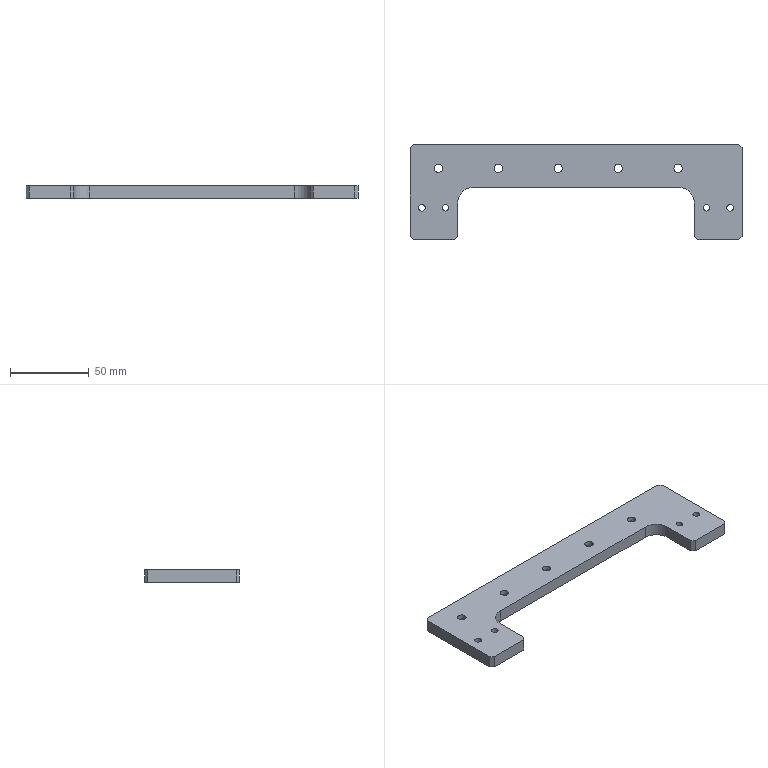Part | STEP file | GLSJ-10-02_default | 1 solid | 51 faces | box 210.5 x 60 x 8 mm | volume 58950 mm3 | cylinder 30 | plane 21 | commonest cylinder face diameters 5.3 x10 10 x10 4.2 x8 20 x2